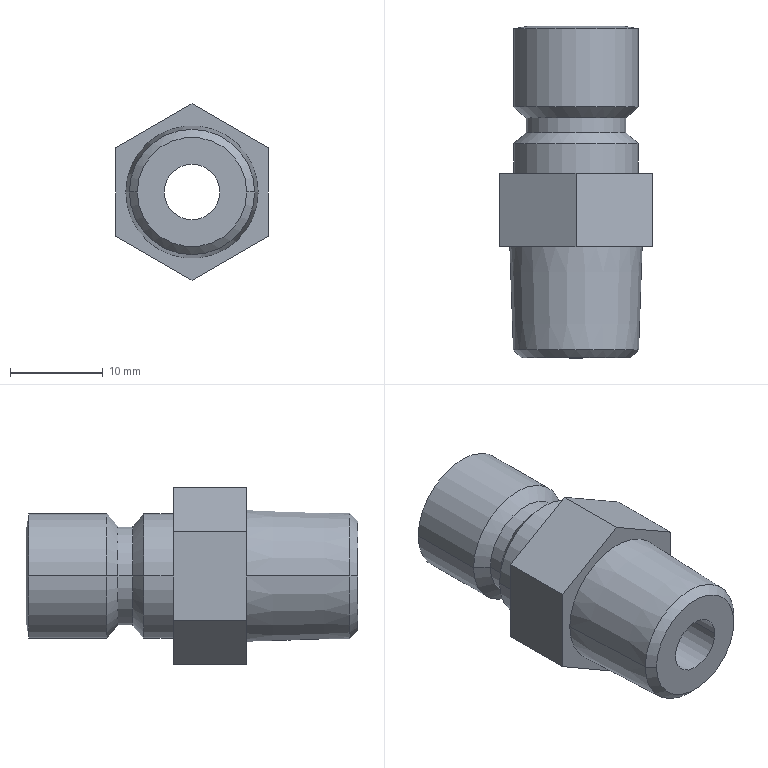Part | Creo | 1 solid | 28 faces | box 16.5 x 35.82 x 19.053 mm | volume 4772 mm3 | plane 10 | cone 10 | cylinder 8 | commonest cylinder face diameters 13.49 x4 6 x2 10.76 x2
STEP:
#1=CARTESIAN_POINT('',(0.,0.,0.));
#2=DIRECTION('',(0.,0.,1.));
#3=DIRECTION('',(1.,0.,0.));
#4=AXIS2_PLACEMENT_3D('',#1,#2,#3);
#5=CARTESIAN_POINT('',(36.045,238.,-1.767));
#6=VERTEX_POINT('',#5);
#7=CARTESIAN_POINT('',(47.855,238.,-1.767));
#8=VERTEX_POINT('',#7);
#9=CARTESIAN_POINT('',(41.95,238.,-1.767));
#10=DIRECTION('',(0.,-1.,0.));
#11=DIRECTION('',(-1.,0.,0.));
#12=AXIS2_PLACEMENT_3D('',#9,#10,#11);
#13=CIRCLE('',#12,5.905);
#14=EDGE_CURVE('',#6,#8,#13,.T.);
#15=ORIENTED_EDGE('',*,*,#14,.F.);
#16=CARTESIAN_POINT('',(41.95,238.,-1.767));
#17=DIRECTION('',(0.,-1.,0.));
#18=DIRECTION('',(1.,0.,0.));
#19=AXIS2_PLACEMENT_3D('',#16,#17,#18);
#20=CIRCLE('',#19,5.905);
#21=EDGE_CURVE('',#8,#6,#20,.T.);
#22=ORIENTED_EDGE('',*,*,#21,.F.);
#23=EDGE_LOOP('',(#15,#22));
#24=FACE_OUTER_BOUND('',#23,.F.);
#25=CARTESIAN_POINT('',(38.95,238.,-1.767));
#26=VERTEX_POINT('',#25);
#27=CARTESIAN_POINT('',(44.95,238.,-1.767));
#28=VERTEX_POINT('',#27);
#29=CARTESIAN_POINT('',(41.95,238.,-1.767));
#30=DIRECTION('',(0.,1.,0.));
#31=DIRECTION('',(-1.,0.,0.));
#32=AXIS2_PLACEMENT_3D('',#29,#30,#31);
#33=CIRCLE('',#32,3.);
#34=EDGE_CURVE('',#26,#28,#33,.T.);
#35=ORIENTED_EDGE('',*,*,#34,.F.);
#36=CARTESIAN_POINT('',(41.95,238.,-1.767));
#37=DIRECTION('',(0.,1.,0.));
#38=DIRECTION('',(1.,0.,0.));
#39=AXIS2_PLACEMENT_3D('',#36,#37,#38);
#40=CIRCLE('',#39,3.);
#41=EDGE_CURVE('',#28,#26,#40,.T.);
#42=ORIENTED_EDGE('',*,*,#41,.F.);
#43=EDGE_LOOP('',(#35,#42));
#44=FACE_BOUND('',#43,.F.);
#45=CARTESIAN_POINT('',(41.95,238.,-1.767));
#46=DIRECTION('',(0.,-1.,0.));
#47=DIRECTION('',(0.,0.,1.));
#48=AXIS2_PLACEMENT_3D('',#45,#46,#47);
#49=PLANE('',#48);
#50=ADVANCED_FACE('',(#24,#44),#49,.T.);
#51=ORIENTED_EDGE('',*,*,#14,.T.);
#52=CARTESIAN_POINT('',(48.71,238.86,-1.767));
#53=VERTEX_POINT('',#52);
#54=CARTESIAN_POINT('',(47.855,238.,-1.767));
#55=DIRECTION('',(0.705,0.7092,0.));
#56=VECTOR('',#55,1.213);
#57=LINE('',#54,#56);
#58=EDGE_CURVE('',#8,#53,#57,.T.);
#59=ORIENTED_EDGE('',*,*,#58,.T.);
#60=CARTESIAN_POINT('',(35.19,238.86,-1.767));
#61=VERTEX_POINT('',#60);
#62=CARTESIAN_POINT('',(41.95,238.86,-1.767));
#63=DIRECTION('',(0.,1.,0.));
#64=DIRECTION('',(1.,0.,0.));
#65=AXIS2_PLACEMENT_3D('',#62,#63,#64);
#66=CIRCLE('',#65,6.76);
#67=EDGE_CURVE('',#53,#61,#66,.T.);
#68=ORIENTED_EDGE('',*,*,#67,.T.);
#69=CARTESIAN_POINT('',(36.045,238.,-1.767));
#70=DIRECTION('',(-0.705,0.7092,0.));
#71=VECTOR('',#70,1.213);
#72=LINE('',#69,#71);
#73=EDGE_CURVE('',#6,#61,#72,.T.);
#74=ORIENTED_EDGE('',*,*,#73,.F.);
#75=EDGE_LOOP('',(#51,#59,#68,#74));
#76=FACE_OUTER_BOUND('',#75,.F.);
#77=CARTESIAN_POINT('',(41.95,238.43,-1.767));
#78=DIRECTION('',(0.,1.,0.));
#79=DIRECTION('',(-1.,0.,0.));
#80=AXIS2_PLACEMENT_3D('',#77,#78,#79);
#81=CONICAL_SURFACE('',#80,6.332,44.833);
#82=ADVANCED_FACE('',(#76),#81,.T.);
#83=ORIENTED_EDGE('',*,*,#21,.T.);
#84=ORIENTED_EDGE('',*,*,#73,.T.);
#85=CARTESIAN_POINT('',(41.95,238.86,-1.767));
#86=DIRECTION('',(0.,1.,0.));
#87=DIRECTION('',(-1.,0.,0.));
#88=AXIS2_PLACEMENT_3D('',#85,#86,#87);
#89=CIRCLE('',#88,6.76);
#90=EDGE_CURVE('',#61,#53,#89,.T.);
#91=ORIENTED_EDGE('',*,*,#90,.T.);
#92=ORIENTED_EDGE('',*,*,#58,.F.);
#93=EDGE_LOOP('',(#83,#84,#91,#92));
#94=FACE_OUTER_BOUND('',#93,.F.);
#95=CARTESIAN_POINT('',(41.95,238.43,-1.767));
#96=DIRECTION('',(0.,1.,0.));
#97=DIRECTION('',(-1.,0.,0.));
#98=AXIS2_PLACEMENT_3D('',#95,#96,#97);
#99=CONICAL_SURFACE('',#98,6.332,44.833);
#100=ADVANCED_FACE('',(#94),#99,.T.);
#101=ORIENTED_EDGE('',*,*,#90,.F.);
#102=CARTESIAN_POINT('',(34.81,250.,-1.767));
#103=VERTEX_POINT('',#102);
#104=CARTESIAN_POINT('',(35.19,238.86,-1.767));
#105=DIRECTION('',(-0.03409,0.9994,0.));
#106=VECTOR('',#105,11.146);
#107=LINE('',#104,#106);
#108=EDGE_CURVE('',#61,#103,#107,.T.);
#109=ORIENTED_EDGE('',*,*,#108,.T.);
#110=CARTESIAN_POINT('',(49.09,250.,-1.767));
#111=VERTEX_POINT('',#110);
#112=CARTESIAN_POINT('',(41.95,250.,-1.767));
#113=DIRECTION('',(0.,1.,0.));
#114=DIRECTION('',(-1.,0.,0.));
#115=AXIS2_PLACEMENT_3D('',#112,#113,#114);
#116=CIRCLE('',#115,7.14);
#117=EDGE_CURVE('',#103,#111,#116,.T.);
#118=ORIENTED_EDGE('',*,*,#117,.T.);
#119=CARTESIAN_POINT('',(48.71,238.86,-1.767));
#120=DIRECTION('',(0.03409,0.9994,0.));
#121=VECTOR('',#120,11.146);
#122=LINE('',#119,#121);
#123=EDGE_CURVE('',#53,#111,#122,.T.);
#124=ORIENTED_EDGE('',*,*,#123,.F.);
#125=EDGE_LOOP('',(#101,#109,#118,#124));
#126=FACE_OUTER_BOUND('',#125,.F.);
#127=CARTESIAN_POINT('',(41.95,244.43,-1.767));
#128=DIRECTION('',(0.,1.,0.));
#129=DIRECTION('',(-1.,0.,0.));
#130=AXIS2_PLACEMENT_3D('',#127,#128,#129);
#131=CONICAL_SURFACE('',#130,6.95,1.954);
#132=ADVANCED_FACE('',(#126),#131,.T.);
#133=ORIENTED_EDGE('',*,*,#67,.F.);
#134=ORIENTED_EDGE('',*,*,#123,.T.);
#135=CARTESIAN_POINT('',(41.95,250.,-1.767));
#136=DIRECTION('',(0.,1.,0.));
#137=DIRECTION('',(1.,0.,0.));
#138=AXIS2_PLACEMENT_3D('',#135,#136,#137);
#139=CIRCLE('',#138,7.14);
#140=EDGE_CURVE('',#111,#103,#139,.T.);
#141=ORIENTED_EDGE('',*,*,#140,.T.);
#142=ORIENTED_EDGE('',*,*,#108,.F.);
#143=EDGE_LOOP('',(#133,#134,#141,#142));
#144=FACE_OUTER_BOUND('',#143,.F.);
#145=CARTESIAN_POINT('',(41.95,244.43,-1.767));
#146=DIRECTION('',(0.,1.,0.));
#147=DIRECTION('',(-1.,0.,0.));
#148=AXIS2_PLACEMENT_3D('',#145,#146,#147);
#149=CONICAL_SURFACE('',#148,6.95,1.954);
#150=ADVANCED_FACE('',(#144),#149,.T.);
#151=CARTESIAN_POINT('',(41.95,250.,-11.293));
#152=VERTEX_POINT('',#151);
#153=CARTESIAN_POINT('',(50.2,250.,-6.53));
#154=VERTEX_POINT('',#153);
#155=CARTESIAN_POINT('',(41.95,250.,-11.293));
#156=DIRECTION('',(0.866,0.,0.5));
#157=VECTOR('',#156,9.526);
#158=LINE('',#155,#157);
#159=EDGE_CURVE('',#152,#154,#158,.T.);
#160=ORIENTED_EDGE('',*,*,#159,.F.);
#161=CARTESIAN_POINT('',(33.7,250.,-6.53));
#162=VERTEX_POINT('',#161);
#163=CARTESIAN_POINT('',(33.7,250.,-6.53));
#164=DIRECTION('',(0.866,0.,-0.5));
#165=VECTOR('',#164,9.526);
#166=LINE('',#163,#165);
#167=EDGE_CURVE('',#162,#152,#166,.T.);
#168=ORIENTED_EDGE('',*,*,#167,.F.);
#169=CARTESIAN_POINT('',(33.7,250.,2.996));
#170=VERTEX_POINT('',#169);
#171=CARTESIAN_POINT('',(33.7,250.,-6.53));
#172=DIRECTION('',(0.,0.,1.));
#173=VECTOR('',#172,9.526);
#174=LINE('',#171,#173);
#175=EDGE_CURVE('',#162,#170,#174,.T.);
#176=ORIENTED_EDGE('',*,*,#175,.T.);
#177=CARTESIAN_POINT('',(41.95,250.,7.759));
#178=VERTEX_POINT('',#177);
#179=CARTESIAN_POINT('',(41.95,250.,7.759));
#180=DIRECTION('',(-0.866,0.,-0.5));
#181=VECTOR('',#180,9.526);
#182=LINE('',#179,#181);
#183=EDGE_CURVE('',#178,#170,#182,.T.);
#184=ORIENTED_EDGE('',*,*,#183,.F.);
#185=CARTESIAN_POINT('',(50.2,250.,2.996));
#186=VERTEX_POINT('',#185);
#187=CARTESIAN_POINT('',(50.2,250.,2.996));
#188=DIRECTION('',(-0.866,0.,0.5));
#189=VECTOR('',#188,9.526);
#190=LINE('',#187,#189);
#191=EDGE_CURVE('',#186,#178,#190,.T.);
#192=ORIENTED_EDGE('',*,*,#191,.F.);
#193=CARTESIAN_POINT('',(50.2,250.,2.996));
#194=DIRECTION('',(0.,0.,-1.));
#195=VECTOR('',#194,9.526);
#196=LINE('',#193,#195);
#197=EDGE_CURVE('',#186,#154,#196,.T.);
#198=ORIENTED_EDGE('',*,*,#197,.T.);
#199=EDGE_LOOP('',(#160,#168,#176,#184,#192,#198));
#200=FACE_OUTER_BOUND('',#199,.F.);
#201=ORIENTED_EDGE('',*,*,#117,.F.);
#202=ORIENTED_EDGE('',*,*,#140,.F.);
#203=EDGE_LOOP('',(#201,#202));
#204=FACE_BOUND('',#203,.F.);
#205=CARTESIAN_POINT('',(41.95,250.,-1.767));
#206=DIRECTION('',(0.,-1.,0.));
#207=DIRECTION('',(0.,0.,1.));
#208=AXIS2_PLACEMENT_3D('',#205,#206,#207);
#209=PLANE('',#208);
#210=ADVANCED_FACE('',(#200,#204),#209,.T.);
#211=CARTESIAN_POINT('',(50.2,257.94,-6.53));
#212=VERTEX_POINT('',#211);
#213=CARTESIAN_POINT('',(41.95,257.94,-11.293));
#214=VERTEX_POINT('',#213);
#215=CARTESIAN_POINT('',(50.2,257.94,-6.53));
#216=DIRECTION('',(-0.866,0.,-0.5));
#217=VECTOR('',#216,9.526);
#218=LINE('',#215,#217);
#219=EDGE_CURVE('',#212,#214,#218,.T.);
#220=ORIENTED_EDGE('',*,*,#219,.T.);
#221=CARTESIAN_POINT('',(41.95,257.94,-11.293));
#222=DIRECTION('',(0.,-1.,0.));
#223=VECTOR('',#222,7.94);
#224=LINE('',#221,#223);
#225=EDGE_CURVE('',#214,#152,#224,.T.);
#226=ORIENTED_EDGE('',*,*,#225,.T.);
#227=ORIENTED_EDGE('',*,*,#159,.T.);
#228=CARTESIAN_POINT('',(50.2,257.94,-6.53));
#229=DIRECTION('',(0.,-1.,0.));
#230=VECTOR('',#229,7.94);
#231=LINE('',#228,#230);
#232=EDGE_CURVE('',#212,#154,#231,.T.);
#233=ORIENTED_EDGE('',*,*,#232,.F.);
#234=EDGE_LOOP('',(#220,#226,#227,#233));
#235=FACE_OUTER_BOUND('',#234,.F.);
#236=CARTESIAN_POINT('',(46.075,253.97,-8.912));
#237=DIRECTION('',(0.5,0.,-0.866));
#238=DIRECTION('',(-0.866,0.,-0.5));
#239=AXIS2_PLACEMENT_3D('',#236,#237,#238);
#240=PLANE('',#239);
#241=ADVANCED_FACE('',(#235),#240,.T.);
#242=CARTESIAN_POINT('',(33.7,257.94,-6.53));
#243=VERTEX_POINT('',#242);
#244=CARTESIAN_POINT('',(33.7,257.94,2.996));
#245=VERTEX_POINT('',#244);
#246=CARTESIAN_POINT('',(33.7,257.94,-6.53));
#247=DIRECTION('',(0.,0.,1.));
#248=VECTOR('',#247,9.526);
#249=LINE('',#246,#248);
#250=EDGE_CURVE('',#243,#245,#249,.T.);
#251=ORIENTED_EDGE('',*,*,#250,.F.);
#252=CARTESIAN_POINT('',(41.95,257.94,-11.293));
#253=DIRECTION('',(-0.866,0.,0.5));
#254=VECTOR('',#253,9.526);
#255=LINE('',#252,#254);
#256=EDGE_CURVE('',#214,#243,#255,.T.);
#257=ORIENTED_EDGE('',*,*,#256,.F.);
#258=ORIENTED_EDGE('',*,*,#219,.F.);
#259=CARTESIAN_POINT('',(50.2,257.94,2.996));
#260=VERTEX_POINT('',#259);
#261=CARTESIAN_POINT('',(50.2,257.94,2.996));
#262=DIRECTION('',(0.,0.,-1.));
#263=VECTOR('',#262,9.526);
#264=LINE('',#261,#263);
#265=EDGE_CURVE('',#260,#212,#264,.T.);
#266=ORIENTED_EDGE('',*,*,#265,.F.);
#267=CARTESIAN_POINT('',(41.95,257.94,7.759));
#268=VERTEX_POINT('',#267);
#269=CARTESIAN_POINT('',(41.95,257.94,7.759));
#270=DIRECTION('',(0.866,0.,-0.5));
#271=VECTOR('',#270,9.526);
#272=LINE('',#269,#271);
#273=EDGE_CURVE('',#268,#260,#272,.T.);
#274=ORIENTED_EDGE('',*,*,#273,.F.);
#275=CARTESIAN_POINT('',(33.7,257.94,2.996));
#276=DIRECTION('',(0.866,0.,0.5));
#277=VECTOR('',#276,9.526);
#278=LINE('',#275,#277);
#279=EDGE_CURVE('',#245,#268,#278,.T.);
#280=ORIENTED_EDGE('',*,*,#279,.F.);
#281=EDGE_LOOP('',(#251,#257,#258,#266,#274,#280));
#282=FACE_OUTER_BOUND('',#281,.F.);
#283=CARTESIAN_POINT('',(35.205,257.94,-1.767));
#284=VERTEX_POINT('',#283);
#285=CARTESIAN_POINT('',(48.695,257.94,-1.767));
#286=VERTEX_POINT('',#285);
#287=CARTESIAN_POINT('',(41.95,257.94,-1.767));
#288=DIRECTION('',(0.,-1.,0.));
#289=DIRECTION('',(-1.,0.,0.));
#290=AXIS2_PLACEMENT_3D('',#287,#288,#289);
#291=CIRCLE('',#290,6.745);
#292=EDGE_CURVE('',#284,#286,#291,.T.);
#293=ORIENTED_EDGE('',*,*,#292,.F.);
#294=CARTESIAN_POINT('',(41.95,257.94,-1.767));
#295=DIRECTION('',(0.,-1.,0.));
#296=DIRECTION('',(1.,0.,0.));
#297=AXIS2_PLACEMENT_3D('',#294,#295,#296);
#298=CIRCLE('',#297,6.745);
#299=EDGE_CURVE('',#286,#284,#298,.T.);
#300=ORIENTED_EDGE('',*,*,#299,.F.);
#301=EDGE_LOOP('',(#293,#300));
#302=FACE_BOUND('',#301,.F.);
#303=CARTESIAN_POINT('',(41.95,257.94,-1.767));
#304=DIRECTION('',(0.,1.,0.));
#305=DIRECTION('',(0.,0.,-1.));
#306=AXIS2_PLACEMENT_3D('',#303,#304,#305);
#307=PLANE('',#306);
#308=ADVANCED_FACE('',(#282,#302),#307,.T.);
#309=CARTESIAN_POINT('',(48.695,261.12,-1.767));
#310=VERTEX_POINT('',#309);
#311=CARTESIAN_POINT('',(35.205,261.12,-1.767));
#312=VERTEX_POINT('',#311);
#313=CARTESIAN_POINT('',(41.95,261.12,-1.767));
#314=DIRECTION('',(0.,1.,0.));
#315=DIRECTION('',(1.,0.,0.));
#316=AXIS2_PLACEMENT_3D('',#313,#314,#315);
#317=CIRCLE('',#316,6.745);
#318=EDGE_CURVE('',#310,#312,#317,.T.);
#319=ORIENTED_EDGE('',*,*,#318,.T.);
#320=CARTESIAN_POINT('',(35.205,257.94,-1.767));
#321=DIRECTION('',(0.,1.,0.));
#322=VECTOR('',#321,3.18);
#323=LINE('',#320,#322);
#324=EDGE_CURVE('',#284,#312,#323,.T.);
#325=ORIENTED_EDGE('',*,*,#324,.F.);
#326=ORIENTED_EDGE('',*,*,#292,.T.);
#327=CARTESIAN_POINT('',(48.695,257.94,-1.767));
#328=DIRECTION('',(0.,1.,0.));
#329=VECTOR('',#328,3.18);
#330=LINE('',#327,#329);
#331=EDGE_CURVE('',#286,#310,#330,.T.);
#332=ORIENTED_EDGE('',*,*,#331,.T.);
#333=EDGE_LOOP('',(#319,#325,#326,#332));
#334=FACE_OUTER_BOUND('',#333,.F.);
#335=CARTESIAN_POINT('',(41.95,257.94,-1.767));
#336=DIRECTION('',(0.,1.,0.));
#337=DIRECTION('',(-1.,0.,0.));
#338=AXIS2_PLACEMENT_3D('',#335,#336,#337);
#339=CYLINDRICAL_SURFACE('',#338,6.745);
#340=ADVANCED_FACE('',(#334),#339,.T.);
#341=CARTESIAN_POINT('',(36.57,262.31,-1.767));
#342=VERTEX_POINT('',#341);
#343=CARTESIAN_POINT('',(47.33,262.31,-1.767));
#344=VERTEX_POINT('',#343);
#345=CARTESIAN_POINT('',(41.95,262.31,-1.767));
#346=DIRECTION('',(0.,-1.,0.));
#347=DIRECTION('',(-1.,0.,0.));
#348=AXIS2_PLACEMENT_3D('',#345,#346,#347);
#349=CIRCLE('',#348,5.38);
#350=EDGE_CURVE('',#342,#344,#349,.T.);
#351=ORIENTED_EDGE('',*,*,#350,.F.);
#352=CARTESIAN_POINT('',(36.57,262.31,-1.767));
#353=DIRECTION('',(-0.7538,-0.6571,0.));
#354=VECTOR('',#353,1.811);
#355=LINE('',#352,#354);
#356=EDGE_CURVE('',#342,#312,#355,.T.);
#357=ORIENTED_EDGE('',*,*,#356,.T.);
#358=ORIENTED_EDGE('',*,*,#318,.F.);
#359=CARTESIAN_POINT('',(47.33,262.31,-1.767));
#360=DIRECTION('',(0.7538,-0.6571,0.));
#361=VECTOR('',#360,1.811);
#362=LINE('',#359,#361);
#363=EDGE_CURVE('',#344,#310,#362,.T.);
#364=ORIENTED_EDGE('',*,*,#363,.F.);
#365=EDGE_LOOP('',(#351,#357,#358,#364));
#366=FACE_OUTER_BOUND('',#365,.F.);
#367=CARTESIAN_POINT('',(41.95,261.715,-1.767));
#368=DIRECTION('',(0.,-1.,0.));
#369=DIRECTION('',(1.,0.,0.));
#370=AXIS2_PLACEMENT_3D('',#367,#368,#369);
#371=CONICAL_SURFACE('',#370,6.062,48.918);
#372=ADVANCED_FACE('',(#366),#371,.T.);
#373=CARTESIAN_POINT('',(47.33,263.9,-1.767));
#374=VERTEX_POINT('',#373);
#375=CARTESIAN_POINT('',(36.57,263.9,-1.767));
#376=VERTEX_POINT('',#375);
#377=CARTESIAN_POINT('',(41.95,263.9,-1.767));
#378=DIRECTION('',(0.,1.,0.));
#379=DIRECTION('',(1.,0.,0.));
#380=AXIS2_PLACEMENT_3D('',#377,#378,#379);
#381=CIRCLE('',#380,5.38);
#382=EDGE_CURVE('',#374,#376,#381,.T.);
#383=ORIENTED_EDGE('',*,*,#382,.T.);
#384=CARTESIAN_POINT('',(36.57,262.31,-1.767));
#385=DIRECTION('',(0.,1.,0.));
#386=VECTOR('',#385,1.59);
#387=LINE('',#384,#386);
#388=EDGE_CURVE('',#342,#376,#387,.T.);
#389=ORIENTED_EDGE('',*,*,#388,.F.);
#390=ORIENTED_EDGE('',*,*,#350,.T.);
#391=CARTESIAN_POINT('',(47.33,262.31,-1.767));
#392=DIRECTION('',(0.,1.,0.));
#393=VECTOR('',#392,1.59);
#394=LINE('',#391,#393);
#395=EDGE_CURVE('',#344,#374,#394,.T.);
#396=ORIENTED_EDGE('',*,*,#395,.T.);
#397=EDGE_LOOP('',(#383,#389,#390,#396));
#398=FACE_OUTER_BOUND('',#397,.F.);
#399=CARTESIAN_POINT('',(41.95,262.31,-1.767));
#400=DIRECTION('',(0.,1.,0.));
#401=DIRECTION('',(-1.,0.,0.));
#402=AXIS2_PLACEMENT_3D('',#399,#400,#401);
#403=CYLINDRICAL_SURFACE('',#402,5.38);
#404=ADVANCED_FACE('',(#398),#403,.T.);
#405=ORIENTED_EDGE('',*,*,#382,.F.);
#406=CARTESIAN_POINT('',(48.695,265.09,-1.767));
#407=VERTEX_POINT('',#406);
#408=CARTESIAN_POINT('',(47.33,263.9,-1.767));
#409=DIRECTION('',(0.7538,0.6571,0.));
#410=VECTOR('',#409,1.811);
#411=LINE('',#408,#410);
#412=EDGE_CURVE('',#374,#407,#411,.T.);
#413=ORIENTED_EDGE('',*,*,#412,.T.);
#414=CARTESIAN_POINT('',(35.205,265.09,-1.767));
#415=VERTEX_POINT('',#414);
#416=CARTESIAN_POINT('',(41.95,265.09,-1.767));
#417=DIRECTION('',(0.,-1.,0.));
#418=DIRECTION('',(-1.,0.,0.));
#419=AXIS2_PLACEMENT_3D('',#416,#417,#418);
#420=CIRCLE('',#419,6.745);
#421=EDGE_CURVE('',#415,#407,#420,.T.);
#422=ORIENTED_EDGE('',*,*,#421,.F.);
#423=CARTESIAN_POINT('',(36.57,263.9,-1.767));
#424=DIRECTION('',(-0.7538,0.6571,0.));
#425=VECTOR('',#424,1.811);
#426=LINE('',#423,#425);
#427=EDGE_CURVE('',#376,#415,#426,.T.);
#428=ORIENTED_EDGE('',*,*,#427,.F.);
#429=EDGE_LOOP('',(#405,#413,#422,#428));
#430=FACE_OUTER_BOUND('',#429,.F.);
#431=CARTESIAN_POINT('',(41.95,264.495,-1.767));
#432=DIRECTION('',(0.,1.,0.));
#433=DIRECTION('',(-1.,0.,0.));
#434=AXIS2_PLACEMENT_3D('',#431,#432,#433);
#435=CONICAL_SURFACE('',#434,6.062,48.918);
#436=ADVANCED_FACE('',(#430),#435,.T.);
#437=CARTESIAN_POINT('',(41.95,263.9,-1.767));
#438=DIRECTION('',(0.,1.,0.));
#439=DIRECTION('',(-1.,0.,0.));
#440=AXIS2_PLACEMENT_3D('',#437,#438,#439);
#441=CIRCLE('',#440,5.38);
#442=EDGE_CURVE('',#376,#374,#441,.T.);
#443=ORIENTED_EDGE('',*,*,#442,.F.);
#444=ORIENTED_EDGE('',*,*,#427,.T.);
#445=CARTESIAN_POINT('',(41.95,265.09,-1.767));
#446=DIRECTION('',(0.,-1.,0.));
#447=DIRECTION('',(1.,0.,0.));
#448=AXIS2_PLACEMENT_3D('',#445,#446,#447);
#449=CIRCLE('',#448,6.745);
#450=EDGE_CURVE('',#407,#415,#449,.T.);
#451=ORIENTED_EDGE('',*,*,#450,.F.);
#452=ORIENTED_EDGE('',*,*,#412,.F.);
#453=EDGE_LOOP('',(#443,#444,#451,#452));
#454=FACE_OUTER_BOUND('',#453,.F.);
#455=CARTESIAN_POINT('',(41.95,264.495,-1.767));
#456=DIRECTION('',(0.,1.,0.));
#457=DIRECTION('',(-1.,0.,0.));
#458=AXIS2_PLACEMENT_3D('',#455,#456,#457);
#459=CONICAL_SURFACE('',#458,6.062,48.918);
#460=ADVANCED_FACE('',(#454),#459,.T.);
#461=ORIENTED_EDGE('',*,*,#442,.T.);
#462=ORIENTED_EDGE('',*,*,#395,.F.);
#463=CARTESIAN_POINT('',(41.95,262.31,-1.767));
#464=DIRECTION('',(0.,-1.,0.));
#465=DIRECTION('',(1.,0.,0.));
#466=AXIS2_PLACEMENT_3D('',#463,#464,#465);
#467=CIRCLE('',#466,5.38);
#468=EDGE_CURVE('',#344,#342,#467,.T.);
#469=ORIENTED_EDGE('',*,*,#468,.T.);
#470=ORIENTED_EDGE('',*,*,#388,.T.);
#471=EDGE_LOOP('',(#461,#462,#469,#470));
#472=FACE_OUTER_BOUND('',#471,.F.);
#473=CARTESIAN_POINT('',(41.95,262.31,-1.767));
#474=DIRECTION('',(0.,1.,0.));
#475=DIRECTION('',(-1.,0.,0.));
#476=AXIS2_PLACEMENT_3D('',#473,#474,#475);
#477=CYLINDRICAL_SURFACE('',#476,5.38);
#478=ADVANCED_FACE('',(#472),#477,.T.);
#479=ORIENTED_EDGE('',*,*,#468,.F.);
#480=ORIENTED_EDGE('',*,*,#363,.T.);
#481=CARTESIAN_POINT('',(41.95,261.12,-1.767));
#482=DIRECTION('',(0.,1.,0.));
#483=DIRECTION('',(-1.,0.,0.));
#484=AXIS2_PLACEMENT_3D('',#481,#482,#483);
#485=CIRCLE('',#484,6.745);
#486=EDGE_CURVE('',#312,#310,#485,.T.);
#487=ORIENTED_EDGE('',*,*,#486,.F.);
#488=ORIENTED_EDGE('',*,*,#356,.F.);
#489=EDGE_LOOP('',(#479,#480,#487,#488));
#490=FACE_OUTER_BOUND('',#489,.F.);
#491=CARTESIAN_POINT('',(41.95,261.715,-1.767));
#492=DIRECTION('',(0.,-1.,0.));
#493=DIRECTION('',(1.,0.,0.));
#494=AXIS2_PLACEMENT_3D('',#491,#492,#493);
#495=CONICAL_SURFACE('',#494,6.062,48.918);
#496=ADVANCED_FACE('',(#490),#495,.T.);
#497=ORIENTED_EDGE('',*,*,#486,.T.);
#498=ORIENTED_EDGE('',*,*,#331,.F.);
#499=ORIENTED_EDGE('',*,*,#299,.T.);
#500=ORIENTED_EDGE('',*,*,#324,.T.);
#501=EDGE_LOOP('',(#497,#498,#499,#500));
#502=FACE_OUTER_BOUND('',#501,.F.);
#503=CARTESIAN_POINT('',(41.95,257.94,-1.767));
#504=DIRECTION('',(0.,1.,0.));
#505=DIRECTION('',(-1.,0.,0.));
#506=AXIS2_PLACEMENT_3D('',#503,#504,#505);
#507=CYLINDRICAL_SURFACE('',#506,6.745);
#508=ADVANCED_FACE('',(#502),#507,.T.);
#509=CARTESIAN_POINT('',(35.205,273.54,-1.767));
#510=VERTEX_POINT('',#509);
#511=CARTESIAN_POINT('',(48.695,273.54,-1.767));
#512=VERTEX_POINT('',#511);
#513=CARTESIAN_POINT('',(41.95,273.54,-1.767));
#514=DIRECTION('',(0.,1.,0.));
#515=DIRECTION('',(-1.,0.,0.));
#516=AXIS2_PLACEMENT_3D('',#513,#514,#515);
#517=CIRCLE('',#516,6.745);
#518=EDGE_CURVE('',#510,#512,#517,.T.);
#519=ORIENTED_EDGE('',*,*,#518,.T.);
#520=CARTESIAN_POINT('',(48.695,265.09,-1.767));
#521=DIRECTION('',(0.,1.,0.));
#522=VECTOR('',#521,8.45);
#523=LINE('',#520,#522);
#524=EDGE_CURVE('',#407,#512,#523,.T.);
#525=ORIENTED_EDGE('',*,*,#524,.F.);
#526=ORIENTED_EDGE('',*,*,#450,.T.);
#527=CARTESIAN_POINT('',(35.205,265.09,-1.767));
#528=DIRECTION('',(0.,1.,0.));
#529=VECTOR('',#528,8.45);
#530=LINE('',#527,#529);
#531=EDGE_CURVE('',#415,#510,#530,.T.);
#532=ORIENTED_EDGE('',*,*,#531,.T.);
#533=EDGE_LOOP('',(#519,#525,#526,#532));
#534=FACE_OUTER_BOUND('',#533,.F.);
#535=CARTESIAN_POINT('',(41.95,265.09,-1.767));
#536=DIRECTION('',(0.,1.,0.));
#537=DIRECTION('',(-1.,0.,0.));
#538=AXIS2_PLACEMENT_3D('',#535,#536,#537);
#539=CYLINDRICAL_SURFACE('',#538,6.745);
#540=ADVANCED_FACE('',(#534),#539,.T.);
#541=CARTESIAN_POINT('',(36.95,273.82,-1.767));
#542=VERTEX_POINT('',#541);
#543=CARTESIAN_POINT('',(46.95,273.82,-1.767));
#544=VERTEX_POINT('',#543);
#545=CARTESIAN_POINT('',(41.95,273.82,-1.767));
#546=DIRECTION('',(0.,1.,0.));
#547=DIRECTION('',(-1.,0.,0.));
#548=AXIS2_PLACEMENT_3D('',#545,#546,#547);
#549=CIRCLE('',#548,5.);
#550=EDGE_CURVE('',#542,#544,#549,.T.);
#551=ORIENTED_EDGE('',*,*,#550,.T.);
#552=CARTESIAN_POINT('',(46.95,273.82,-1.767));
#553=DIRECTION('',(0.9874,-0.1584,0.));
#554=VECTOR('',#553,1.767);
#555=LINE('',#552,#554);
#556=EDGE_CURVE('',#544,#512,#555,.T.);
#557=ORIENTED_EDGE('',*,*,#556,.T.);
#558=ORIENTED_EDGE('',*,*,#518,.F.);
#559=CARTESIAN_POINT('',(36.95,273.82,-1.767));
#560=DIRECTION('',(-0.9874,-0.1584,0.));
#561=VECTOR('',#560,1.767);
#562=LINE('',#559,#561);
#563=EDGE_CURVE('',#542,#510,#562,.T.);
#564=ORIENTED_EDGE('',*,*,#563,.F.);
#565=EDGE_LOOP('',(#551,#557,#558,#564));
#566=FACE_OUTER_BOUND('',#565,.F.);
#567=CARTESIAN_POINT('',(41.95,273.68,-1.767));
#568=DIRECTION('',(0.,-1.,0.));
#569=DIRECTION('',(1.,0.,0.));
#570=AXIS2_PLACEMENT_3D('',#567,#568,#569);
#571=CONICAL_SURFACE('',#570,5.872,80.884);
#572=ADVANCED_FACE('',(#566),#571,.T.);
#573=CARTESIAN_POINT('',(41.95,273.82,-1.767));
#574=DIRECTION('',(0.,1.,0.));
#575=DIRECTION('',(1.,0.,0.));
#576=AXIS2_PLACEMENT_3D('',#573,#574,#575);
#577=CIRCLE('',#576,5.);
#578=EDGE_CURVE('',#544,#542,#577,.T.);
#579=ORIENTED_EDGE('',*,*,#578,.F.);
#580=ORIENTED_EDGE('',*,*,#550,.F.);
#581=EDGE_LOOP('',(#579,#580));
#582=FACE_OUTER_BOUND('',#581,.F.);
#583=CARTESIAN_POINT('',(38.95,273.82,-1.767));
#584=VERTEX_POINT('',#583);
#585=CARTESIAN_POINT('',(44.95,273.82,-1.767));
#586=VERTEX_POINT('',#585);
#587=CARTESIAN_POINT('',(41.95,273.82,-1.767));
#588=DIRECTION('',(0.,-1.,0.));
#589=DIRECTION('',(-1.,0.,0.));
#590=AXIS2_PLACEMENT_3D('',#587,#588,#589);
#591=CIRCLE('',#590,3.);
#592=EDGE_CURVE('',#584,#586,#591,.T.);
#593=ORIENTED_EDGE('',*,*,#592,.F.);
#594=CARTESIAN_POINT('',(41.95,273.82,-1.767));
#595=DIRECTION('',(0.,-1.,0.));
#596=DIRECTION('',(1.,0.,0.));
#597=AXIS2_PLACEMENT_3D('',#594,#595,#596);
#598=CIRCLE('',#597,3.);
#599=EDGE_CURVE('',#586,#584,#598,.T.);
#600=ORIENTED_EDGE('',*,*,#599,.F.);
#601=EDGE_LOOP('',(#593,#600));
#602=FACE_BOUND('',#601,.F.);
#603=CARTESIAN_POINT('',(41.95,273.82,-1.767));
#604=DIRECTION('',(0.,1.,0.));
#605=DIRECTION('',(0.,0.,-1.));
#606=AXIS2_PLACEMENT_3D('',#603,#604,#605);
#607=PLANE('',#606);
#608=ADVANCED_FACE('',(#582,#602),#607,.T.);
#609=ORIENTED_EDGE('',*,*,#578,.T.);
#610=ORIENTED_EDGE('',*,*,#563,.T.);
#611=CARTESIAN_POINT('',(41.95,273.54,-1.767));
#612=DIRECTION('',(0.,1.,0.));
#613=DIRECTION('',(1.,0.,0.));
#614=AXIS2_PLACEMENT_3D('',#611,#612,#613);
#615=CIRCLE('',#614,6.745);
#616=EDGE_CURVE('',#512,#510,#615,.T.);
#617=ORIENTED_EDGE('',*,*,#616,.F.);
#618=ORIENTED_EDGE('',*,*,#556,.F.);
#619=EDGE_LOOP('',(#609,#610,#617,#618));
#620=FACE_OUTER_BOUND('',#619,.F.);
#621=CARTESIAN_POINT('',(41.95,273.68,-1.767));
#622=DIRECTION('',(0.,-1.,0.));
#623=DIRECTION('',(1.,0.,0.));
#624=AXIS2_PLACEMENT_3D('',#621,#622,#623);
#625=CONICAL_SURFACE('',#624,5.872,80.884);
#626=ADVANCED_FACE('',(#620),#625,.T.);
#627=ORIENTED_EDGE('',*,*,#616,.T.);
#628=ORIENTED_EDGE('',*,*,#531,.F.);
#629=ORIENTED_EDGE('',*,*,#421,.T.);
#630=ORIENTED_EDGE('',*,*,#524,.T.);
#631=EDGE_LOOP('',(#627,#628,#629,#630));
#632=FACE_OUTER_BOUND('',#631,.F.);
#633=CARTESIAN_POINT('',(41.95,265.09,-1.767));
#634=DIRECTION('',(0.,1.,0.));
#635=DIRECTION('',(-1.,0.,0.));
#636=AXIS2_PLACEMENT_3D('',#633,#634,#635);
#637=CYLINDRICAL_SURFACE('',#636,6.745);
#638=ADVANCED_FACE('',(#632),#637,.T.);
#639=ORIENTED_EDGE('',*,*,#592,.T.);
#640=CARTESIAN_POINT('',(44.95,238.,-1.767));
#641=DIRECTION('',(0.,1.,0.));
#642=VECTOR('',#641,35.82);
#643=LINE('',#640,#642);
#644=EDGE_CURVE('',#28,#586,#643,.T.);
#645=ORIENTED_EDGE('',*,*,#644,.F.);
#646=ORIENTED_EDGE('',*,*,#41,.T.);
#647=CARTESIAN_POINT('',(38.95,238.,-1.767));
#648=DIRECTION('',(0.,1.,0.));
#649=VECTOR('',#648,35.82);
#650=LINE('',#647,#649);
#651=EDGE_CURVE('',#26,#584,#650,.T.);
#652=ORIENTED_EDGE('',*,*,#651,.T.);
#653=EDGE_LOOP('',(#639,#645,#646,#652));
#654=FACE_OUTER_BOUND('',#653,.F.);
#655=CARTESIAN_POINT('',(41.95,238.,-1.767));
#656=DIRECTION('',(0.,1.,0.));
#657=DIRECTION('',(-1.,0.,0.));
#658=AXIS2_PLACEMENT_3D('',#655,#656,#657);
#659=CYLINDRICAL_SURFACE('',#658,3.);
#660=ADVANCED_FACE('',(#654),#659,.F.);
#661=ORIENTED_EDGE('',*,*,#599,.T.);
#662=ORIENTED_EDGE('',*,*,#651,.F.);
#663=ORIENTED_EDGE('',*,*,#34,.T.);
#664=ORIENTED_EDGE('',*,*,#644,.T.);
#665=EDGE_LOOP('',(#661,#662,#663,#664));
#666=FACE_OUTER_BOUND('',#665,.F.);
#667=CARTESIAN_POINT('',(41.95,238.,-1.767));
#668=DIRECTION('',(0.,1.,0.));
#669=DIRECTION('',(-1.,0.,0.));
#670=AXIS2_PLACEMENT_3D('',#667,#668,#669);
#671=CYLINDRICAL_SURFACE('',#670,3.);
#672=ADVANCED_FACE('',(#666),#671,.F.);
#673=ORIENTED_EDGE('',*,*,#250,.T.);
#674=CARTESIAN_POINT('',(33.7,257.94,2.996));
#675=DIRECTION('',(0.,-1.,0.));
#676=VECTOR('',#675,7.94);
#677=LINE('',#674,#676);
#678=EDGE_CURVE('',#245,#170,#677,.T.);
#679=ORIENTED_EDGE('',*,*,#678,.T.);
#680=ORIENTED_EDGE('',*,*,#175,.F.);
#681=CARTESIAN_POINT('',(33.7,257.94,-6.53));
#682=DIRECTION('',(0.,-1.,0.));
#683=VECTOR('',#682,7.94);
#684=LINE('',#681,#683);
#685=EDGE_CURVE('',#243,#162,#684,.T.);
#686=ORIENTED_EDGE('',*,*,#685,.F.);
#687=EDGE_LOOP('',(#673,#679,#680,#686));
#688=FACE_OUTER_BOUND('',#687,.F.);
#689=CARTESIAN_POINT('',(33.7,253.97,-1.767));
#690=DIRECTION('',(-1.,0.,0.));
#691=DIRECTION('',(0.,0.,1.));
#692=AXIS2_PLACEMENT_3D('',#689,#690,#691);
#693=PLANE('',#692);
#694=ADVANCED_FACE('',(#688),#693,.T.);
#695=ORIENTED_EDGE('',*,*,#279,.T.);
#696=CARTESIAN_POINT('',(41.95,257.94,7.759));
#697=DIRECTION('',(0.,-1.,0.));
#698=VECTOR('',#697,7.94);
#699=LINE('',#696,#698);
#700=EDGE_CURVE('',#268,#178,#699,.T.);
#701=ORIENTED_EDGE('',*,*,#700,.T.);
#702=ORIENTED_EDGE('',*,*,#183,.T.);
#703=ORIENTED_EDGE('',*,*,#678,.F.);
#704=EDGE_LOOP('',(#695,#701,#702,#703));
#705=FACE_OUTER_BOUND('',#704,.F.);
#706=CARTESIAN_POINT('',(37.825,253.97,5.378));
#707=DIRECTION('',(-0.5,0.,0.866));
#708=DIRECTION('',(0.866,0.,0.5));
#709=AXIS2_PLACEMENT_3D('',#706,#707,#708);
#710=PLANE('',#709);
#711=ADVANCED_FACE('',(#705),#710,.T.);
#712=ORIENTED_EDGE('',*,*,#273,.T.);
#713=CARTESIAN_POINT('',(50.2,257.94,2.996));
#714=DIRECTION('',(0.,-1.,0.));
#715=VECTOR('',#714,7.94);
#716=LINE('',#713,#715);
#717=EDGE_CURVE('',#260,#186,#716,.T.);
#718=ORIENTED_EDGE('',*,*,#717,.T.);
#719=ORIENTED_EDGE('',*,*,#191,.T.);
#720=ORIENTED_EDGE('',*,*,#700,.F.);
#721=EDGE_LOOP('',(#712,#718,#719,#720));
#722=FACE_OUTER_BOUND('',#721,.F.);
#723=CARTESIAN_POINT('',(46.075,253.97,5.378));
#724=DIRECTION('',(0.5,0.,0.866));
#725=DIRECTION('',(0.866,0.,-0.5));
#726=AXIS2_PLACEMENT_3D('',#723,#724,#725);
#727=PLANE('',#726);
#728=ADVANCED_FACE('',(#722),#727,.T.);
#729=ORIENTED_EDGE('',*,*,#265,.T.);
#730=ORIENTED_EDGE('',*,*,#232,.T.);
#731=ORIENTED_EDGE('',*,*,#197,.F.);
#732=ORIENTED_EDGE('',*,*,#717,.F.);
#733=EDGE_LOOP('',(#729,#730,#731,#732));
#734=FACE_OUTER_BOUND('',#733,.F.);
#735=CARTESIAN_POINT('',(50.2,253.97,-1.767));
#736=DIRECTION('',(1.,0.,0.));
#737=DIRECTION('',(0.,-1.,0.));
#738=AXIS2_PLACEMENT_3D('',#735,#736,#737);
#739=PLANE('',#738);
#740=ADVANCED_FACE('',(#734),#739,.T.);
#741=ORIENTED_EDGE('',*,*,#256,.T.);
#742=ORIENTED_EDGE('',*,*,#685,.T.);
#743=ORIENTED_EDGE('',*,*,#167,.T.);
#744=ORIENTED_EDGE('',*,*,#225,.F.);
#745=EDGE_LOOP('',(#741,#742,#743,#744));
#746=FACE_OUTER_BOUND('',#745,.F.);
#747=CARTESIAN_POINT('',(37.825,253.97,-8.912));
#748=DIRECTION('',(-0.5,0.,-0.866));
#749=DIRECTION('',(-0.866,0.,0.5));
#750=AXIS2_PLACEMENT_3D('',#747,#748,#749);
#751=PLANE('',#750);
#752=ADVANCED_FACE('',(#746),#751,.T.);
#753=CLOSED_SHELL('',(#50,#82,#100,#132,#150,#210,#241,#308,#340,#372,#404,#436,#460,#478,#496,#508,#540,#572,#608,#626,#638,#660,#672,#694,#711,#728,#740,#752));
#754=MANIFOLD_SOLID_BREP('',#753);
#755=(LENGTH_UNIT()NAMED_UNIT(*)SI_UNIT(.MILLI.,.METRE.));
#756=UNCERTAINTY_MEASURE_WITH_UNIT(LENGTH_MEASURE(0.00438),#755,'','');
#757=(NAMED_UNIT(*)PLANE_ANGLE_UNIT()SI_UNIT($,.RADIAN.));
#758=PLANE_ANGLE_MEASURE_WITH_UNIT(PLANE_ANGLE_MEASURE(0.01745),#757);
#759=(CONVERSION_BASED_UNIT('DEGREE',#758)NAMED_UNIT(*)PLANE_ANGLE_UNIT());
#760=(NAMED_UNIT(*)SI_UNIT($,.STERADIAN.)SOLID_ANGLE_UNIT());
#761=(GEOMETRIC_REPRESENTATION_CONTEXT(3)GLOBAL_UNCERTAINTY_ASSIGNED_CONTEXT((#756))GLOBAL_UNIT_ASSIGNED_CONTEXT((#755,#759,#760))REPRESENTATION_CONTEXT('',''));
#762=ADVANCED_BREP_SHAPE_REPRESENTATION('',(#4,#754),#761);